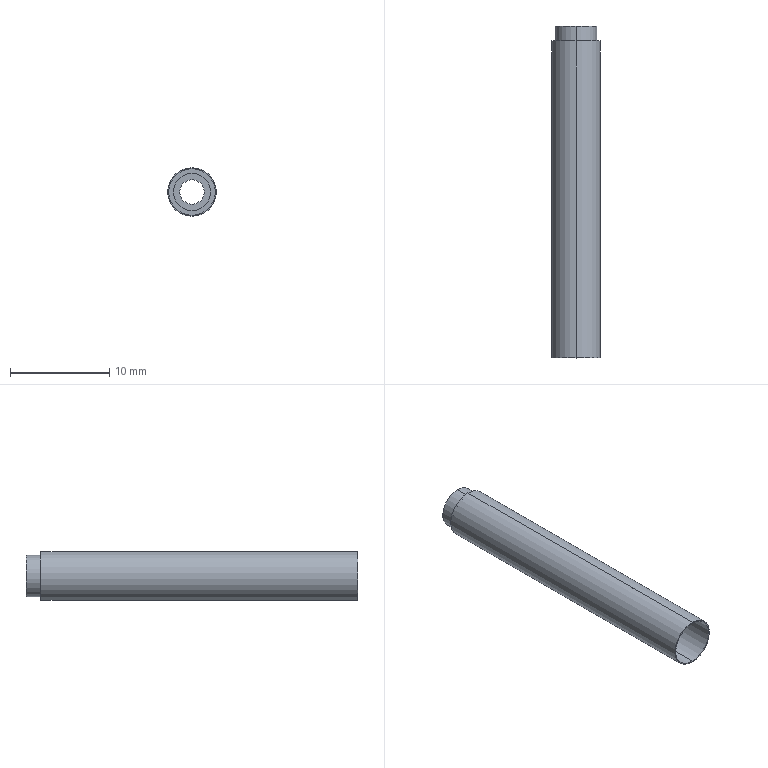Part | SolidWorks | features Revolution 1 | 1 solid | 15 faces | box 4.9 x 33.507 x 4.9 mm | volume 63.209 mm3 | cylinder 10 | plane 5 | commonest cylinder face diameters 2.46 x2 3.768 x2 4.2 x2 4.7 x2 4.9 x2
STEP:
#1=CARTESIAN_POINT('',(0.,29.94,-2.45));
#2=VERTEX_POINT('',#1);
#3=CARTESIAN_POINT('',(0.,29.94,2.45));
#4=VERTEX_POINT('',#3);
#5=CARTESIAN_POINT('',(0.,29.94,0.));
#6=DIRECTION('',(0.,-1.,0.));
#7=DIRECTION('',(0.,0.,-1.));
#8=AXIS2_PLACEMENT_3D('',#5,#6,#7);
#9=CIRCLE('',#8,2.45);
#10=EDGE_CURVE('',#2,#4,#9,.T.);
#11=ORIENTED_EDGE('',*,*,#10,.T.);
#12=CARTESIAN_POINT('',(0.,-2.06,2.45));
#13=VERTEX_POINT('',#12);
#14=CARTESIAN_POINT('',(0.,-5.46,2.45));
#15=DIRECTION('',(0.,-1.,0.));
#16=VECTOR('',#15,1000.);
#17=LINE('',#14,#16);
#18=EDGE_CURVE('',#4,#13,#17,.T.);
#19=ORIENTED_EDGE('',*,*,#18,.T.);
#20=CARTESIAN_POINT('',(0.,-2.06,-2.45));
#21=VERTEX_POINT('',#20);
#22=CARTESIAN_POINT('',(0.,-2.06,0.));
#23=DIRECTION('',(0.,-1.,0.));
#24=DIRECTION('',(0.,0.,-1.));
#25=AXIS2_PLACEMENT_3D('',#22,#23,#24);
#26=CIRCLE('',#25,2.45);
#27=EDGE_CURVE('',#21,#13,#26,.T.);
#28=ORIENTED_EDGE('',*,*,#27,.F.);
#29=CARTESIAN_POINT('',(0.,-5.46,-2.45));
#30=DIRECTION('',(0.,-1.,0.));
#31=VECTOR('',#30,1000.);
#32=LINE('',#29,#31);
#33=EDGE_CURVE('',#2,#21,#32,.T.);
#34=ORIENTED_EDGE('',*,*,#33,.F.);
#35=EDGE_LOOP('',(#11,#19,#28,#34));
#36=FACE_OUTER_BOUND('',#35,.T.);
#37=CARTESIAN_POINT('',(0.,-5.46,0.));
#38=DIRECTION('',(0.,-1.,0.));
#39=DIRECTION('',(0.,0.,-1.));
#40=AXIS2_PLACEMENT_3D('',#37,#38,#39);
#41=CYLINDRICAL_SURFACE('',#40,2.45);
#42=ADVANCED_FACE('',(#36),#41,.T.);
#43=CARTESIAN_POINT('',(0.,31.447,-2.1));
#44=VERTEX_POINT('',#43);
#45=CARTESIAN_POINT('',(0.,31.447,2.1));
#46=VERTEX_POINT('',#45);
#47=CARTESIAN_POINT('',(0.,31.447,0.));
#48=DIRECTION('',(0.,-1.,0.));
#49=DIRECTION('',(0.,0.,-1.));
#50=AXIS2_PLACEMENT_3D('',#47,#48,#49);
#51=CIRCLE('',#50,2.1);
#52=EDGE_CURVE('',#44,#46,#51,.T.);
#53=ORIENTED_EDGE('',*,*,#52,.T.);
#54=CARTESIAN_POINT('',(0.,29.94,2.1));
#55=VERTEX_POINT('',#54);
#56=CARTESIAN_POINT('',(0.,-5.46,2.1));
#57=DIRECTION('',(0.,-1.,0.));
#58=VECTOR('',#57,1000.);
#59=LINE('',#56,#58);
#60=EDGE_CURVE('',#46,#55,#59,.T.);
#61=ORIENTED_EDGE('',*,*,#60,.T.);
#62=CARTESIAN_POINT('',(0.,29.94,-2.1));
#63=VERTEX_POINT('',#62);
#64=CARTESIAN_POINT('',(0.,29.94,0.));
#65=DIRECTION('',(0.,-1.,0.));
#66=DIRECTION('',(0.,0.,-1.));
#67=AXIS2_PLACEMENT_3D('',#64,#65,#66);
#68=CIRCLE('',#67,2.1);
#69=EDGE_CURVE('',#63,#55,#68,.T.);
#70=ORIENTED_EDGE('',*,*,#69,.F.);
#71=CARTESIAN_POINT('',(0.,-5.46,-2.1));
#72=DIRECTION('',(0.,-1.,0.));
#73=VECTOR('',#72,1000.);
#74=LINE('',#71,#73);
#75=EDGE_CURVE('',#44,#63,#74,.T.);
#76=ORIENTED_EDGE('',*,*,#75,.F.);
#77=EDGE_LOOP('',(#53,#61,#70,#76));
#78=FACE_OUTER_BOUND('',#77,.T.);
#79=CARTESIAN_POINT('',(0.,-5.46,0.));
#80=DIRECTION('',(0.,-1.,0.));
#81=DIRECTION('',(0.,0.,-1.));
#82=AXIS2_PLACEMENT_3D('',#79,#80,#81);
#83=CYLINDRICAL_SURFACE('',#82,2.1);
#84=ADVANCED_FACE('',(#78),#83,.T.);
#85=CARTESIAN_POINT('',(0.,31.447,1.23));
#86=VERTEX_POINT('',#85);
#87=CARTESIAN_POINT('',(0.,31.447,-1.23));
#88=VERTEX_POINT('',#87);
#89=CARTESIAN_POINT('',(0.,31.447,0.));
#90=DIRECTION('',(0.,-1.,0.));
#91=DIRECTION('',(0.,0.,-1.));
#92=AXIS2_PLACEMENT_3D('',#89,#90,#91);
#93=CIRCLE('',#92,1.23);
#94=EDGE_CURVE('',#86,#88,#93,.T.);
#95=ORIENTED_EDGE('',*,*,#94,.F.);
#96=CARTESIAN_POINT('',(0.,29.94,1.23));
#97=VERTEX_POINT('',#96);
#98=CARTESIAN_POINT('',(0.,-5.46,1.23));
#99=DIRECTION('',(0.,-1.,0.));
#100=VECTOR('',#99,1000.);
#101=LINE('',#98,#100);
#102=EDGE_CURVE('',#86,#97,#101,.T.);
#103=ORIENTED_EDGE('',*,*,#102,.T.);
#104=CARTESIAN_POINT('',(0.,29.94,-1.23));
#105=VERTEX_POINT('',#104);
#106=CARTESIAN_POINT('',(0.,29.94,0.));
#107=DIRECTION('',(0.,-1.,0.));
#108=DIRECTION('',(0.,0.,-1.));
#109=AXIS2_PLACEMENT_3D('',#106,#107,#108);
#110=CIRCLE('',#109,1.23);
#111=EDGE_CURVE('',#97,#105,#110,.T.);
#112=ORIENTED_EDGE('',*,*,#111,.T.);
#113=CARTESIAN_POINT('',(0.,-5.46,-1.23));
#114=DIRECTION('',(0.,-1.,0.));
#115=VECTOR('',#114,1000.);
#116=LINE('',#113,#115);
#117=EDGE_CURVE('',#88,#105,#116,.T.);
#118=ORIENTED_EDGE('',*,*,#117,.F.);
#119=EDGE_LOOP('',(#95,#103,#112,#118));
#120=FACE_OUTER_BOUND('',#119,.T.);
#121=CARTESIAN_POINT('',(0.,-5.46,0.));
#122=DIRECTION('',(0.,-1.,0.));
#123=DIRECTION('',(0.,0.,-1.));
#124=AXIS2_PLACEMENT_3D('',#121,#122,#123);
#125=CYLINDRICAL_SURFACE('',#124,1.23);
#126=ADVANCED_FACE('',(#120),#125,.F.);
#127=CARTESIAN_POINT('',(0.,29.94,1.884));
#128=VERTEX_POINT('',#127);
#129=CARTESIAN_POINT('',(0.,29.94,-1.884));
#130=VERTEX_POINT('',#129);
#131=CARTESIAN_POINT('',(0.,29.94,0.));
#132=DIRECTION('',(0.,-1.,0.));
#133=DIRECTION('',(0.,0.,-1.));
#134=AXIS2_PLACEMENT_3D('',#131,#132,#133);
#135=CIRCLE('',#134,1.884);
#136=EDGE_CURVE('',#128,#130,#135,.T.);
#137=ORIENTED_EDGE('',*,*,#136,.F.);
#138=CARTESIAN_POINT('',(0.,29.74,1.884));
#139=VERTEX_POINT('',#138);
#140=CARTESIAN_POINT('',(0.,-5.46,1.884));
#141=DIRECTION('',(0.,-1.,0.));
#142=VECTOR('',#141,1000.);
#143=LINE('',#140,#142);
#144=EDGE_CURVE('',#128,#139,#143,.T.);
#145=ORIENTED_EDGE('',*,*,#144,.T.);
#146=CARTESIAN_POINT('',(0.,29.74,-1.884));
#147=VERTEX_POINT('',#146);
#148=CARTESIAN_POINT('',(0.,29.74,0.));
#149=DIRECTION('',(0.,-1.,0.));
#150=DIRECTION('',(0.,0.,-1.));
#151=AXIS2_PLACEMENT_3D('',#148,#149,#150);
#152=CIRCLE('',#151,1.884);
#153=EDGE_CURVE('',#139,#147,#152,.T.);
#154=ORIENTED_EDGE('',*,*,#153,.T.);
#155=CARTESIAN_POINT('',(0.,-5.46,-1.884));
#156=DIRECTION('',(0.,-1.,0.));
#157=VECTOR('',#156,1000.);
#158=LINE('',#155,#157);
#159=EDGE_CURVE('',#130,#147,#158,.T.);
#160=ORIENTED_EDGE('',*,*,#159,.F.);
#161=EDGE_LOOP('',(#137,#145,#154,#160));
#162=FACE_OUTER_BOUND('',#161,.T.);
#163=CARTESIAN_POINT('',(0.,-5.46,0.));
#164=DIRECTION('',(0.,-1.,0.));
#165=DIRECTION('',(0.,0.,-1.));
#166=AXIS2_PLACEMENT_3D('',#163,#164,#165);
#167=CYLINDRICAL_SURFACE('',#166,1.884);
#168=ADVANCED_FACE('',(#162),#167,.F.);
#169=CARTESIAN_POINT('',(0.,29.74,2.35));
#170=VERTEX_POINT('',#169);
#171=CARTESIAN_POINT('',(0.,29.74,-2.35));
#172=VERTEX_POINT('',#171);
#173=CARTESIAN_POINT('',(0.,29.74,0.));
#174=DIRECTION('',(0.,-1.,0.));
#175=DIRECTION('',(0.,0.,-1.));
#176=AXIS2_PLACEMENT_3D('',#173,#174,#175);
#177=CIRCLE('',#176,2.35);
#178=EDGE_CURVE('',#170,#172,#177,.T.);
#179=ORIENTED_EDGE('',*,*,#178,.F.);
#180=CARTESIAN_POINT('',(0.,-2.06,2.35));
#181=VERTEX_POINT('',#180);
#182=CARTESIAN_POINT('',(0.,-5.46,2.35));
#183=DIRECTION('',(0.,-1.,0.));
#184=VECTOR('',#183,1000.);
#185=LINE('',#182,#184);
#186=EDGE_CURVE('',#170,#181,#185,.T.);
#187=ORIENTED_EDGE('',*,*,#186,.T.);
#188=CARTESIAN_POINT('',(0.,-2.06,-2.35));
#189=VERTEX_POINT('',#188);
#190=CARTESIAN_POINT('',(0.,-2.06,0.));
#191=DIRECTION('',(0.,-1.,0.));
#192=DIRECTION('',(0.,0.,-1.));
#193=AXIS2_PLACEMENT_3D('',#190,#191,#192);
#194=CIRCLE('',#193,2.35);
#195=EDGE_CURVE('',#181,#189,#194,.T.);
#196=ORIENTED_EDGE('',*,*,#195,.T.);
#197=CARTESIAN_POINT('',(0.,-5.46,-2.35));
#198=DIRECTION('',(0.,-1.,0.));
#199=VECTOR('',#198,1000.);
#200=LINE('',#197,#199);
#201=EDGE_CURVE('',#172,#189,#200,.T.);
#202=ORIENTED_EDGE('',*,*,#201,.F.);
#203=EDGE_LOOP('',(#179,#187,#196,#202));
#204=FACE_OUTER_BOUND('',#203,.T.);
#205=CARTESIAN_POINT('',(0.,-5.46,0.));
#206=DIRECTION('',(0.,-1.,0.));
#207=DIRECTION('',(0.,0.,-1.));
#208=AXIS2_PLACEMENT_3D('',#205,#206,#207);
#209=CYLINDRICAL_SURFACE('',#208,2.35);
#210=ADVANCED_FACE('',(#204),#209,.F.);
#211=CARTESIAN_POINT('',(0.,-2.06,0.));
#212=DIRECTION('',(0.,-1.,0.));
#213=DIRECTION('',(0.,0.,-1.));
#214=AXIS2_PLACEMENT_3D('',#211,#212,#213);
#215=CIRCLE('',#214,2.35);
#216=EDGE_CURVE('',#189,#181,#215,.T.);
#217=ORIENTED_EDGE('',*,*,#216,.F.);
#218=ORIENTED_EDGE('',*,*,#195,.F.);
#219=EDGE_LOOP('',(#217,#218));
#220=FACE_BOUND('',#219,.T.);
#221=ORIENTED_EDGE('',*,*,#27,.T.);
#222=CARTESIAN_POINT('',(0.,-2.06,0.));
#223=DIRECTION('',(0.,-1.,0.));
#224=DIRECTION('',(0.,0.,-1.));
#225=AXIS2_PLACEMENT_3D('',#222,#223,#224);
#226=CIRCLE('',#225,2.45);
#227=EDGE_CURVE('',#13,#21,#226,.T.);
#228=ORIENTED_EDGE('',*,*,#227,.T.);
#229=EDGE_LOOP('',(#221,#228));
#230=FACE_OUTER_BOUND('',#229,.T.);
#231=CARTESIAN_POINT('',(-2.45,-2.06,0.));
#232=DIRECTION('',(0.,1.,0.));
#233=DIRECTION('',(0.,0.,1.));
#234=AXIS2_PLACEMENT_3D('',#231,#232,#233);
#235=PLANE('',#234);
#236=ADVANCED_FACE('',(#220,#230),#235,.F.);
#237=ORIENTED_EDGE('',*,*,#186,.F.);
#238=CARTESIAN_POINT('',(0.,29.74,0.));
#239=DIRECTION('',(0.,-1.,0.));
#240=DIRECTION('',(0.,0.,-1.));
#241=AXIS2_PLACEMENT_3D('',#238,#239,#240);
#242=CIRCLE('',#241,2.35);
#243=EDGE_CURVE('',#172,#170,#242,.T.);
#244=ORIENTED_EDGE('',*,*,#243,.F.);
#245=ORIENTED_EDGE('',*,*,#201,.T.);
#246=ORIENTED_EDGE('',*,*,#216,.T.);
#247=EDGE_LOOP('',(#237,#244,#245,#246));
#248=FACE_OUTER_BOUND('',#247,.T.);
#249=CARTESIAN_POINT('',(0.,-5.46,0.));
#250=DIRECTION('',(0.,-1.,0.));
#251=DIRECTION('',(0.,0.,-1.));
#252=AXIS2_PLACEMENT_3D('',#249,#250,#251);
#253=CYLINDRICAL_SURFACE('',#252,2.35);
#254=ADVANCED_FACE('',(#248),#253,.F.);
#255=CARTESIAN_POINT('',(0.,29.74,0.));
#256=DIRECTION('',(0.,-1.,0.));
#257=DIRECTION('',(0.,0.,-1.));
#258=AXIS2_PLACEMENT_3D('',#255,#256,#257);
#259=CIRCLE('',#258,1.884);
#260=EDGE_CURVE('',#147,#139,#259,.T.);
#261=ORIENTED_EDGE('',*,*,#260,.F.);
#262=ORIENTED_EDGE('',*,*,#153,.F.);
#263=EDGE_LOOP('',(#261,#262));
#264=FACE_BOUND('',#263,.T.);
#265=ORIENTED_EDGE('',*,*,#243,.T.);
#266=ORIENTED_EDGE('',*,*,#178,.T.);
#267=EDGE_LOOP('',(#265,#266));
#268=FACE_OUTER_BOUND('',#267,.T.);
#269=CARTESIAN_POINT('',(-2.35,29.74,0.));
#270=DIRECTION('',(0.,1.,0.));
#271=DIRECTION('',(0.,0.,1.));
#272=AXIS2_PLACEMENT_3D('',#269,#270,#271);
#273=PLANE('',#272);
#274=ADVANCED_FACE('',(#264,#268),#273,.F.);
#275=ORIENTED_EDGE('',*,*,#144,.F.);
#276=CARTESIAN_POINT('',(0.,29.94,0.));
#277=DIRECTION('',(0.,-1.,0.));
#278=DIRECTION('',(0.,0.,-1.));
#279=AXIS2_PLACEMENT_3D('',#276,#277,#278);
#280=CIRCLE('',#279,1.884);
#281=EDGE_CURVE('',#130,#128,#280,.T.);
#282=ORIENTED_EDGE('',*,*,#281,.F.);
#283=ORIENTED_EDGE('',*,*,#159,.T.);
#284=ORIENTED_EDGE('',*,*,#260,.T.);
#285=EDGE_LOOP('',(#275,#282,#283,#284));
#286=FACE_OUTER_BOUND('',#285,.T.);
#287=CARTESIAN_POINT('',(0.,-5.46,0.));
#288=DIRECTION('',(0.,-1.,0.));
#289=DIRECTION('',(0.,0.,-1.));
#290=AXIS2_PLACEMENT_3D('',#287,#288,#289);
#291=CYLINDRICAL_SURFACE('',#290,1.884);
#292=ADVANCED_FACE('',(#286),#291,.F.);
#293=CARTESIAN_POINT('',(0.,29.94,0.));
#294=DIRECTION('',(0.,-1.,0.));
#295=DIRECTION('',(0.,0.,-1.));
#296=AXIS2_PLACEMENT_3D('',#293,#294,#295);
#297=CIRCLE('',#296,1.23);
#298=EDGE_CURVE('',#105,#97,#297,.T.);
#299=ORIENTED_EDGE('',*,*,#298,.F.);
#300=ORIENTED_EDGE('',*,*,#111,.F.);
#301=EDGE_LOOP('',(#299,#300));
#302=FACE_BOUND('',#301,.T.);
#303=ORIENTED_EDGE('',*,*,#281,.T.);
#304=ORIENTED_EDGE('',*,*,#136,.T.);
#305=EDGE_LOOP('',(#303,#304));
#306=FACE_OUTER_BOUND('',#305,.T.);
#307=CARTESIAN_POINT('',(-1.884,29.94,0.));
#308=DIRECTION('',(0.,1.,0.));
#309=DIRECTION('',(0.,0.,1.));
#310=AXIS2_PLACEMENT_3D('',#307,#308,#309);
#311=PLANE('',#310);
#312=ADVANCED_FACE('',(#302,#306),#311,.F.);
#313=ORIENTED_EDGE('',*,*,#102,.F.);
#314=CARTESIAN_POINT('',(0.,31.447,0.));
#315=DIRECTION('',(0.,-1.,0.));
#316=DIRECTION('',(0.,0.,-1.));
#317=AXIS2_PLACEMENT_3D('',#314,#315,#316);
#318=CIRCLE('',#317,1.23);
#319=EDGE_CURVE('',#88,#86,#318,.T.);
#320=ORIENTED_EDGE('',*,*,#319,.F.);
#321=ORIENTED_EDGE('',*,*,#117,.T.);
#322=ORIENTED_EDGE('',*,*,#298,.T.);
#323=EDGE_LOOP('',(#313,#320,#321,#322));
#324=FACE_OUTER_BOUND('',#323,.T.);
#325=CARTESIAN_POINT('',(0.,-5.46,0.));
#326=DIRECTION('',(0.,-1.,0.));
#327=DIRECTION('',(0.,0.,-1.));
#328=AXIS2_PLACEMENT_3D('',#325,#326,#327);
#329=CYLINDRICAL_SURFACE('',#328,1.23);
#330=ADVANCED_FACE('',(#324),#329,.F.);
#331=ORIENTED_EDGE('',*,*,#52,.F.);
#332=CARTESIAN_POINT('',(0.,31.447,0.));
#333=DIRECTION('',(0.,-1.,0.));
#334=DIRECTION('',(0.,0.,-1.));
#335=AXIS2_PLACEMENT_3D('',#332,#333,#334);
#336=CIRCLE('',#335,2.1);
#337=EDGE_CURVE('',#46,#44,#336,.T.);
#338=ORIENTED_EDGE('',*,*,#337,.F.);
#339=EDGE_LOOP('',(#331,#338));
#340=FACE_OUTER_BOUND('',#339,.T.);
#341=ORIENTED_EDGE('',*,*,#319,.T.);
#342=ORIENTED_EDGE('',*,*,#94,.T.);
#343=EDGE_LOOP('',(#341,#342));
#344=FACE_BOUND('',#343,.T.);
#345=CARTESIAN_POINT('',(-2.1,31.447,0.));
#346=DIRECTION('',(0.,-1.,0.));
#347=DIRECTION('',(0.,0.,-1.));
#348=AXIS2_PLACEMENT_3D('',#345,#346,#347);
#349=PLANE('',#348);
#350=ADVANCED_FACE('',(#340,#344),#349,.F.);
#351=ORIENTED_EDGE('',*,*,#60,.F.);
#352=ORIENTED_EDGE('',*,*,#337,.T.);
#353=ORIENTED_EDGE('',*,*,#75,.T.);
#354=CARTESIAN_POINT('',(0.,29.94,0.));
#355=DIRECTION('',(0.,-1.,0.));
#356=DIRECTION('',(0.,0.,-1.));
#357=AXIS2_PLACEMENT_3D('',#354,#355,#356);
#358=CIRCLE('',#357,2.1);
#359=EDGE_CURVE('',#55,#63,#358,.T.);
#360=ORIENTED_EDGE('',*,*,#359,.F.);
#361=EDGE_LOOP('',(#351,#352,#353,#360));
#362=FACE_OUTER_BOUND('',#361,.T.);
#363=CARTESIAN_POINT('',(0.,-5.46,0.));
#364=DIRECTION('',(0.,-1.,0.));
#365=DIRECTION('',(0.,0.,-1.));
#366=AXIS2_PLACEMENT_3D('',#363,#364,#365);
#367=CYLINDRICAL_SURFACE('',#366,2.1);
#368=ADVANCED_FACE('',(#362),#367,.T.);
#369=ORIENTED_EDGE('',*,*,#10,.F.);
#370=CARTESIAN_POINT('',(0.,29.94,0.));
#371=DIRECTION('',(0.,-1.,0.));
#372=DIRECTION('',(0.,0.,-1.));
#373=AXIS2_PLACEMENT_3D('',#370,#371,#372);
#374=CIRCLE('',#373,2.45);
#375=EDGE_CURVE('',#4,#2,#374,.T.);
#376=ORIENTED_EDGE('',*,*,#375,.F.);
#377=EDGE_LOOP('',(#369,#376));
#378=FACE_OUTER_BOUND('',#377,.T.);
#379=ORIENTED_EDGE('',*,*,#69,.T.);
#380=ORIENTED_EDGE('',*,*,#359,.T.);
#381=EDGE_LOOP('',(#379,#380));
#382=FACE_BOUND('',#381,.T.);
#383=CARTESIAN_POINT('',(-2.1,29.94,0.));
#384=DIRECTION('',(0.,-1.,0.));
#385=DIRECTION('',(0.,0.,-1.));
#386=AXIS2_PLACEMENT_3D('',#383,#384,#385);
#387=PLANE('',#386);
#388=ADVANCED_FACE('',(#378,#382),#387,.F.);
#389=ORIENTED_EDGE('',*,*,#18,.F.);
#390=ORIENTED_EDGE('',*,*,#375,.T.);
#391=ORIENTED_EDGE('',*,*,#33,.T.);
#392=ORIENTED_EDGE('',*,*,#227,.F.);
#393=EDGE_LOOP('',(#389,#390,#391,#392));
#394=FACE_OUTER_BOUND('',#393,.T.);
#395=CARTESIAN_POINT('',(0.,-5.46,0.));
#396=DIRECTION('',(0.,-1.,0.));
#397=DIRECTION('',(0.,0.,-1.));
#398=AXIS2_PLACEMENT_3D('',#395,#396,#397);
#399=CYLINDRICAL_SURFACE('',#398,2.45);
#400=ADVANCED_FACE('',(#394),#399,.T.);
#401=CLOSED_SHELL('',(#42,#84,#126,#168,#210,#236,#254,#274,#292,#312,#330,#350,#368,#388,#400));
#402=MANIFOLD_SOLID_BREP('',#401);
#403=CARTESIAN_POINT('',(0.,0.,0.));
#404=DIRECTION('',(0.,0.,1.));
#405=DIRECTION('',(1.,0.,0.));
#406=AXIS2_PLACEMENT_3D('',#403,#404,#405);
#407=(LENGTH_UNIT()NAMED_UNIT(*)SI_UNIT(.MILLI.,.METRE.));
#408=UNCERTAINTY_MEASURE_WITH_UNIT(LENGTH_MEASURE(0.00001),#407,'','');
#409=(NAMED_UNIT(*)PLANE_ANGLE_UNIT()SI_UNIT($,.RADIAN.));
#410=(NAMED_UNIT(*)SI_UNIT($,.STERADIAN.)SOLID_ANGLE_UNIT());
#411=(GEOMETRIC_REPRESENTATION_CONTEXT(3)GLOBAL_UNCERTAINTY_ASSIGNED_CONTEXT((#408))GLOBAL_UNIT_ASSIGNED_CONTEXT((#407,#409,#410))REPRESENTATION_CONTEXT('',''));
#412=ADVANCED_BREP_SHAPE_REPRESENTATION('',(#402,#406),#411);